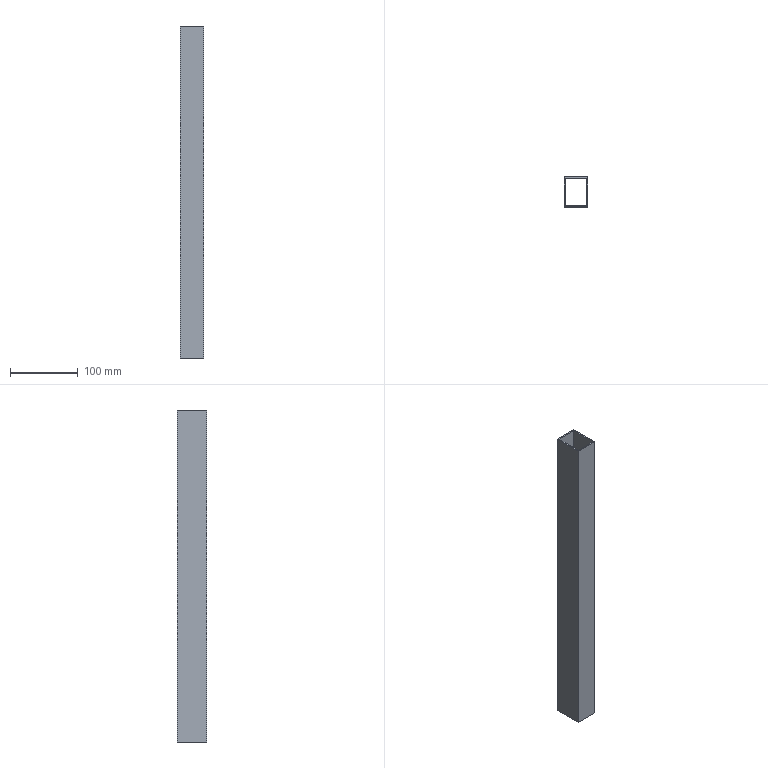Part | SolidWorks | features Extrusion 1 | 1 solid | 10 faces | box 35 x 44 x 488.489 mm | volume 146547 mm3 | plane 10
STEP:
#1=CARTESIAN_POINT('',(-17.5,-22.,488.489));
#2=VERTEX_POINT('',#1);
#3=CARTESIAN_POINT('',(17.5,-22.,488.489));
#4=VERTEX_POINT('',#3);
#5=CARTESIAN_POINT('',(-17.5,-22.,488.489));
#6=DIRECTION('',(1.,0.,0.));
#7=VECTOR('',#6,1000.);
#8=LINE('',#5,#7);
#9=EDGE_CURVE('',#2,#4,#8,.T.);
#10=ORIENTED_EDGE('',*,*,#9,.F.);
#11=CARTESIAN_POINT('',(-17.5,-22.,0.));
#12=VERTEX_POINT('',#11);
#13=CARTESIAN_POINT('',(-17.5,-22.,544.712));
#14=DIRECTION('',(0.,0.,-1.));
#15=VECTOR('',#14,1000.);
#16=LINE('',#13,#15);
#17=EDGE_CURVE('',#2,#12,#16,.T.);
#18=ORIENTED_EDGE('',*,*,#17,.T.);
#19=CARTESIAN_POINT('',(17.5,-22.,0.));
#20=VERTEX_POINT('',#19);
#21=CARTESIAN_POINT('',(-17.5,-22.,0.));
#22=DIRECTION('',(1.,0.,0.));
#23=VECTOR('',#22,1000.);
#24=LINE('',#21,#23);
#25=EDGE_CURVE('',#12,#20,#24,.T.);
#26=ORIENTED_EDGE('',*,*,#25,.T.);
#27=CARTESIAN_POINT('',(17.5,-22.,544.712));
#28=DIRECTION('',(0.,0.,-1.));
#29=VECTOR('',#28,1000.);
#30=LINE('',#27,#29);
#31=EDGE_CURVE('',#4,#20,#30,.T.);
#32=ORIENTED_EDGE('',*,*,#31,.F.);
#33=EDGE_LOOP('',(#10,#18,#26,#32));
#34=FACE_OUTER_BOUND('',#33,.T.);
#35=CARTESIAN_POINT('',(-17.5,-22.,544.712));
#36=DIRECTION('',(0.,1.,0.));
#37=DIRECTION('',(0.,0.,1.));
#38=AXIS2_PLACEMENT_3D('',#35,#36,#37);
#39=PLANE('',#38);
#40=ADVANCED_FACE('',(#34),#39,.F.);
#41=CARTESIAN_POINT('',(-17.5,22.,488.489));
#42=VERTEX_POINT('',#41);
#43=CARTESIAN_POINT('',(-17.5,-22.,488.489));
#44=DIRECTION('',(0.,-1.,0.));
#45=VECTOR('',#44,1000.);
#46=LINE('',#43,#45);
#47=EDGE_CURVE('',#42,#2,#46,.T.);
#48=ORIENTED_EDGE('',*,*,#47,.F.);
#49=CARTESIAN_POINT('',(-17.5,22.,0.));
#50=VERTEX_POINT('',#49);
#51=CARTESIAN_POINT('',(-17.5,22.,544.712));
#52=DIRECTION('',(0.,0.,-1.));
#53=VECTOR('',#52,1000.);
#54=LINE('',#51,#53);
#55=EDGE_CURVE('',#42,#50,#54,.T.);
#56=ORIENTED_EDGE('',*,*,#55,.T.);
#57=CARTESIAN_POINT('',(-17.5,-22.,0.));
#58=DIRECTION('',(0.,-1.,0.));
#59=VECTOR('',#58,1000.);
#60=LINE('',#57,#59);
#61=EDGE_CURVE('',#50,#12,#60,.T.);
#62=ORIENTED_EDGE('',*,*,#61,.T.);
#63=ORIENTED_EDGE('',*,*,#17,.F.);
#64=EDGE_LOOP('',(#48,#56,#62,#63));
#65=FACE_OUTER_BOUND('',#64,.T.);
#66=CARTESIAN_POINT('',(-17.5,-22.,544.712));
#67=DIRECTION('',(1.,0.,0.));
#68=DIRECTION('',(0.,1.,0.));
#69=AXIS2_PLACEMENT_3D('',#66,#67,#68);
#70=PLANE('',#69);
#71=ADVANCED_FACE('',(#65),#70,.F.);
#72=CARTESIAN_POINT('',(17.5,22.,488.489));
#73=VERTEX_POINT('',#72);
#74=CARTESIAN_POINT('',(-17.5,22.,488.489));
#75=DIRECTION('',(-1.,0.,0.));
#76=VECTOR('',#75,1000.);
#77=LINE('',#74,#76);
#78=EDGE_CURVE('',#73,#42,#77,.T.);
#79=ORIENTED_EDGE('',*,*,#78,.F.);
#80=CARTESIAN_POINT('',(17.5,22.,0.));
#81=VERTEX_POINT('',#80);
#82=CARTESIAN_POINT('',(17.5,22.,544.712));
#83=DIRECTION('',(0.,0.,-1.));
#84=VECTOR('',#83,1000.);
#85=LINE('',#82,#84);
#86=EDGE_CURVE('',#73,#81,#85,.T.);
#87=ORIENTED_EDGE('',*,*,#86,.T.);
#88=CARTESIAN_POINT('',(-17.5,22.,0.));
#89=DIRECTION('',(-1.,0.,0.));
#90=VECTOR('',#89,1000.);
#91=LINE('',#88,#90);
#92=EDGE_CURVE('',#81,#50,#91,.T.);
#93=ORIENTED_EDGE('',*,*,#92,.T.);
#94=ORIENTED_EDGE('',*,*,#55,.F.);
#95=EDGE_LOOP('',(#79,#87,#93,#94));
#96=FACE_OUTER_BOUND('',#95,.T.);
#97=CARTESIAN_POINT('',(-17.5,22.,544.712));
#98=DIRECTION('',(0.,-1.,0.));
#99=DIRECTION('',(1.,0.,0.));
#100=AXIS2_PLACEMENT_3D('',#97,#98,#99);
#101=PLANE('',#100);
#102=ADVANCED_FACE('',(#96),#101,.F.);
#103=CARTESIAN_POINT('',(17.5,-22.,488.489));
#104=DIRECTION('',(0.,1.,0.));
#105=VECTOR('',#104,1000.);
#106=LINE('',#103,#105);
#107=EDGE_CURVE('',#4,#73,#106,.T.);
#108=ORIENTED_EDGE('',*,*,#107,.F.);
#109=ORIENTED_EDGE('',*,*,#31,.T.);
#110=CARTESIAN_POINT('',(17.5,-22.,0.));
#111=DIRECTION('',(0.,1.,0.));
#112=VECTOR('',#111,1000.);
#113=LINE('',#110,#112);
#114=EDGE_CURVE('',#20,#81,#113,.T.);
#115=ORIENTED_EDGE('',*,*,#114,.T.);
#116=ORIENTED_EDGE('',*,*,#86,.F.);
#117=EDGE_LOOP('',(#108,#109,#115,#116));
#118=FACE_OUTER_BOUND('',#117,.T.);
#119=CARTESIAN_POINT('',(17.5,-22.,544.712));
#120=DIRECTION('',(-1.,0.,0.));
#121=DIRECTION('',(0.,-1.,0.));
#122=AXIS2_PLACEMENT_3D('',#119,#120,#121);
#123=PLANE('',#122);
#124=ADVANCED_FACE('',(#118),#123,.F.);
#125=ORIENTED_EDGE('',*,*,#114,.F.);
#126=ORIENTED_EDGE('',*,*,#25,.F.);
#127=ORIENTED_EDGE('',*,*,#61,.F.);
#128=ORIENTED_EDGE('',*,*,#92,.F.);
#129=EDGE_LOOP('',(#125,#126,#127,#128));
#130=FACE_OUTER_BOUND('',#129,.T.);
#131=CARTESIAN_POINT('',(15.5,20.,0.));
#132=VERTEX_POINT('',#131);
#133=CARTESIAN_POINT('',(-15.5,20.,0.));
#134=VERTEX_POINT('',#133);
#135=CARTESIAN_POINT('',(-15.5,20.,0.));
#136=DIRECTION('',(-1.,0.,0.));
#137=VECTOR('',#136,1000.);
#138=LINE('',#135,#137);
#139=EDGE_CURVE('',#132,#134,#138,.T.);
#140=ORIENTED_EDGE('',*,*,#139,.T.);
#141=CARTESIAN_POINT('',(-15.5,-20.,0.));
#142=VERTEX_POINT('',#141);
#143=CARTESIAN_POINT('',(-15.5,-20.,0.));
#144=DIRECTION('',(0.,-1.,0.));
#145=VECTOR('',#144,1000.);
#146=LINE('',#143,#145);
#147=EDGE_CURVE('',#134,#142,#146,.T.);
#148=ORIENTED_EDGE('',*,*,#147,.T.);
#149=CARTESIAN_POINT('',(15.5,-20.,0.));
#150=VERTEX_POINT('',#149);
#151=CARTESIAN_POINT('',(-15.5,-20.,0.));
#152=DIRECTION('',(1.,0.,0.));
#153=VECTOR('',#152,1000.);
#154=LINE('',#151,#153);
#155=EDGE_CURVE('',#142,#150,#154,.T.);
#156=ORIENTED_EDGE('',*,*,#155,.T.);
#157=CARTESIAN_POINT('',(15.5,-20.,0.));
#158=DIRECTION('',(0.,1.,0.));
#159=VECTOR('',#158,1000.);
#160=LINE('',#157,#159);
#161=EDGE_CURVE('',#150,#132,#160,.T.);
#162=ORIENTED_EDGE('',*,*,#161,.T.);
#163=EDGE_LOOP('',(#140,#148,#156,#162));
#164=FACE_BOUND('',#163,.T.);
#165=CARTESIAN_POINT('',(0.,0.,0.));
#166=DIRECTION('',(0.,0.,-1.));
#167=DIRECTION('',(-1.,0.,0.));
#168=AXIS2_PLACEMENT_3D('',#165,#166,#167);
#169=PLANE('',#168);
#170=ADVANCED_FACE('',(#130,#164),#169,.T.);
#171=CARTESIAN_POINT('',(15.5,20.,488.489));
#172=VERTEX_POINT('',#171);
#173=CARTESIAN_POINT('',(15.5,20.,544.712));
#174=DIRECTION('',(0.,0.,-1.));
#175=VECTOR('',#174,1000.);
#176=LINE('',#173,#175);
#177=EDGE_CURVE('',#172,#132,#176,.T.);
#178=ORIENTED_EDGE('',*,*,#177,.F.);
#179=CARTESIAN_POINT('',(-15.5,20.,488.489));
#180=VERTEX_POINT('',#179);
#181=CARTESIAN_POINT('',(-15.5,20.,488.489));
#182=DIRECTION('',(-1.,0.,0.));
#183=VECTOR('',#182,1000.);
#184=LINE('',#181,#183);
#185=EDGE_CURVE('',#172,#180,#184,.T.);
#186=ORIENTED_EDGE('',*,*,#185,.T.);
#187=CARTESIAN_POINT('',(-15.5,20.,544.712));
#188=DIRECTION('',(0.,0.,-1.));
#189=VECTOR('',#188,1000.);
#190=LINE('',#187,#189);
#191=EDGE_CURVE('',#180,#134,#190,.T.);
#192=ORIENTED_EDGE('',*,*,#191,.T.);
#193=ORIENTED_EDGE('',*,*,#139,.F.);
#194=EDGE_LOOP('',(#178,#186,#192,#193));
#195=FACE_OUTER_BOUND('',#194,.T.);
#196=CARTESIAN_POINT('',(-15.5,20.,544.712));
#197=DIRECTION('',(0.,-1.,0.));
#198=DIRECTION('',(1.,0.,0.));
#199=AXIS2_PLACEMENT_3D('',#196,#197,#198);
#200=PLANE('',#199);
#201=ADVANCED_FACE('',(#195),#200,.T.);
#202=CARTESIAN_POINT('',(15.5,-20.,488.489));
#203=VERTEX_POINT('',#202);
#204=CARTESIAN_POINT('',(15.5,-20.,544.712));
#205=DIRECTION('',(0.,0.,-1.));
#206=VECTOR('',#205,1000.);
#207=LINE('',#204,#206);
#208=EDGE_CURVE('',#203,#150,#207,.T.);
#209=ORIENTED_EDGE('',*,*,#208,.F.);
#210=CARTESIAN_POINT('',(15.5,-20.,488.489));
#211=DIRECTION('',(0.,1.,0.));
#212=VECTOR('',#211,1000.);
#213=LINE('',#210,#212);
#214=EDGE_CURVE('',#203,#172,#213,.T.);
#215=ORIENTED_EDGE('',*,*,#214,.T.);
#216=ORIENTED_EDGE('',*,*,#177,.T.);
#217=ORIENTED_EDGE('',*,*,#161,.F.);
#218=EDGE_LOOP('',(#209,#215,#216,#217));
#219=FACE_OUTER_BOUND('',#218,.T.);
#220=CARTESIAN_POINT('',(15.5,-20.,544.712));
#221=DIRECTION('',(-1.,0.,0.));
#222=DIRECTION('',(0.,-1.,0.));
#223=AXIS2_PLACEMENT_3D('',#220,#221,#222);
#224=PLANE('',#223);
#225=ADVANCED_FACE('',(#219),#224,.T.);
#226=CARTESIAN_POINT('',(-15.5,-20.,488.489));
#227=VERTEX_POINT('',#226);
#228=CARTESIAN_POINT('',(-15.5,-20.,544.712));
#229=DIRECTION('',(0.,0.,-1.));
#230=VECTOR('',#229,1000.);
#231=LINE('',#228,#230);
#232=EDGE_CURVE('',#227,#142,#231,.T.);
#233=ORIENTED_EDGE('',*,*,#232,.F.);
#234=CARTESIAN_POINT('',(-15.5,-20.,488.489));
#235=DIRECTION('',(1.,0.,0.));
#236=VECTOR('',#235,1000.);
#237=LINE('',#234,#236);
#238=EDGE_CURVE('',#227,#203,#237,.T.);
#239=ORIENTED_EDGE('',*,*,#238,.T.);
#240=ORIENTED_EDGE('',*,*,#208,.T.);
#241=ORIENTED_EDGE('',*,*,#155,.F.);
#242=EDGE_LOOP('',(#233,#239,#240,#241));
#243=FACE_OUTER_BOUND('',#242,.T.);
#244=CARTESIAN_POINT('',(-15.5,-20.,544.712));
#245=DIRECTION('',(0.,1.,0.));
#246=DIRECTION('',(0.,0.,1.));
#247=AXIS2_PLACEMENT_3D('',#244,#245,#246);
#248=PLANE('',#247);
#249=ADVANCED_FACE('',(#243),#248,.T.);
#250=ORIENTED_EDGE('',*,*,#191,.F.);
#251=CARTESIAN_POINT('',(-15.5,-20.,488.489));
#252=DIRECTION('',(0.,-1.,0.));
#253=VECTOR('',#252,1000.);
#254=LINE('',#251,#253);
#255=EDGE_CURVE('',#180,#227,#254,.T.);
#256=ORIENTED_EDGE('',*,*,#255,.T.);
#257=ORIENTED_EDGE('',*,*,#232,.T.);
#258=ORIENTED_EDGE('',*,*,#147,.F.);
#259=EDGE_LOOP('',(#250,#256,#257,#258));
#260=FACE_OUTER_BOUND('',#259,.T.);
#261=CARTESIAN_POINT('',(-15.5,-20.,544.712));
#262=DIRECTION('',(1.,0.,0.));
#263=DIRECTION('',(0.,0.,-1.));
#264=AXIS2_PLACEMENT_3D('',#261,#262,#263);
#265=PLANE('',#264);
#266=ADVANCED_FACE('',(#260),#265,.T.);
#267=ORIENTED_EDGE('',*,*,#185,.F.);
#268=ORIENTED_EDGE('',*,*,#214,.F.);
#269=ORIENTED_EDGE('',*,*,#238,.F.);
#270=ORIENTED_EDGE('',*,*,#255,.F.);
#271=EDGE_LOOP('',(#267,#268,#269,#270));
#272=FACE_BOUND('',#271,.T.);
#273=ORIENTED_EDGE('',*,*,#107,.T.);
#274=ORIENTED_EDGE('',*,*,#78,.T.);
#275=ORIENTED_EDGE('',*,*,#47,.T.);
#276=ORIENTED_EDGE('',*,*,#9,.T.);
#277=EDGE_LOOP('',(#273,#274,#275,#276));
#278=FACE_OUTER_BOUND('',#277,.T.);
#279=CARTESIAN_POINT('',(382.045,26.825,488.489));
#280=DIRECTION('',(0.,0.,1.));
#281=DIRECTION('',(1.,0.,0.));
#282=AXIS2_PLACEMENT_3D('',#279,#280,#281);
#283=PLANE('',#282);
#284=ADVANCED_FACE('',(#272,#278),#283,.T.);
#285=CLOSED_SHELL('',(#40,#71,#102,#124,#170,#201,#225,#249,#266,#284));
#286=MANIFOLD_SOLID_BREP('',#285);
#287=CARTESIAN_POINT('',(0.,0.,0.));
#288=DIRECTION('',(0.,0.,1.));
#289=DIRECTION('',(1.,0.,0.));
#290=AXIS2_PLACEMENT_3D('',#287,#288,#289);
#291=(LENGTH_UNIT()NAMED_UNIT(*)SI_UNIT(.MILLI.,.METRE.));
#292=UNCERTAINTY_MEASURE_WITH_UNIT(LENGTH_MEASURE(0.00001),#291,'','');
#293=(NAMED_UNIT(*)PLANE_ANGLE_UNIT()SI_UNIT($,.RADIAN.));
#294=(NAMED_UNIT(*)SI_UNIT($,.STERADIAN.)SOLID_ANGLE_UNIT());
#295=(GEOMETRIC_REPRESENTATION_CONTEXT(3)GLOBAL_UNCERTAINTY_ASSIGNED_CONTEXT((#292))GLOBAL_UNIT_ASSIGNED_CONTEXT((#291,#293,#294))REPRESENTATION_CONTEXT('',''));
#296=ADVANCED_BREP_SHAPE_REPRESENTATION('',(#286,#290),#295);